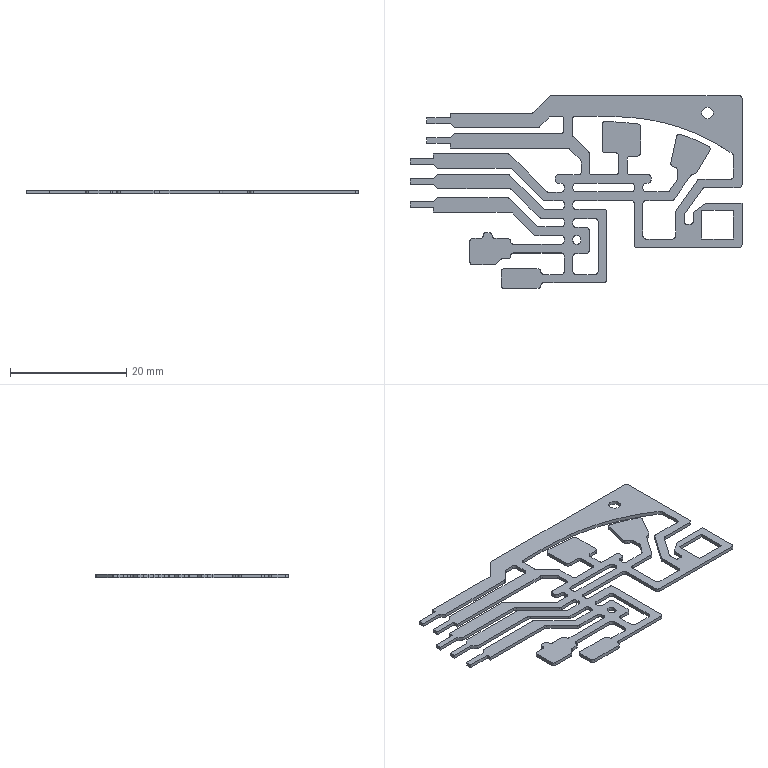Part | NX | features BREP 1 | 1 solid | 267 faces | box 57.003 x 33.1 x 0.6 mm | volume 492.533 mm3 | plane 146 | cylinder 121 | commonest cylinder face diameters 1 x115 2 x1 69.173 x1 72.496 x1 72.701 x1 163.294 x1